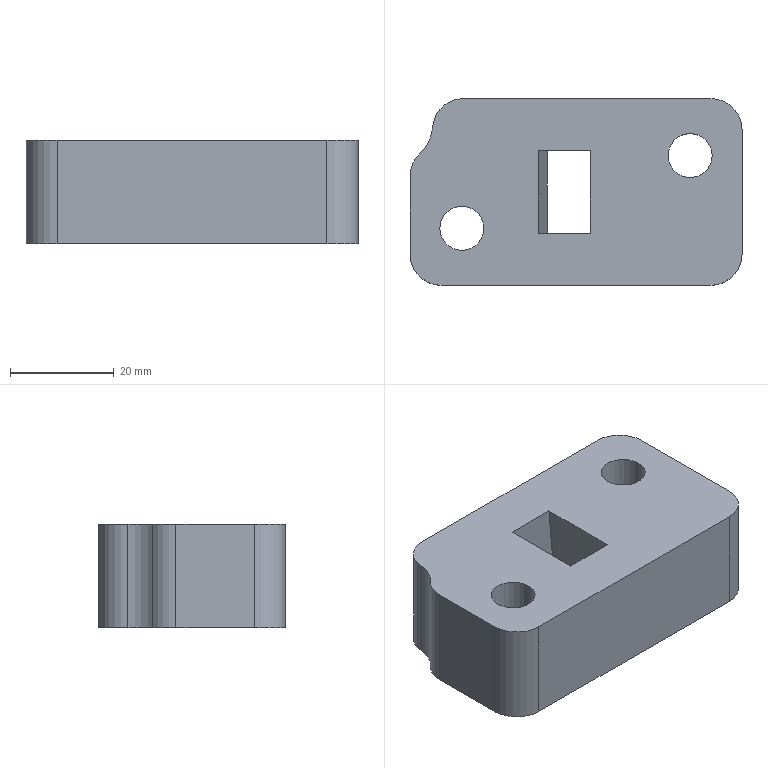Part | STEP file | solid 102 | 1 solid | 36 faces | box 64 x 36 x 20 mm | volume 37344 mm3 | plane 20 | cylinder 10 | other 6 | commonest cylinder face diameters 12 x5 14 x3 8.5 x2